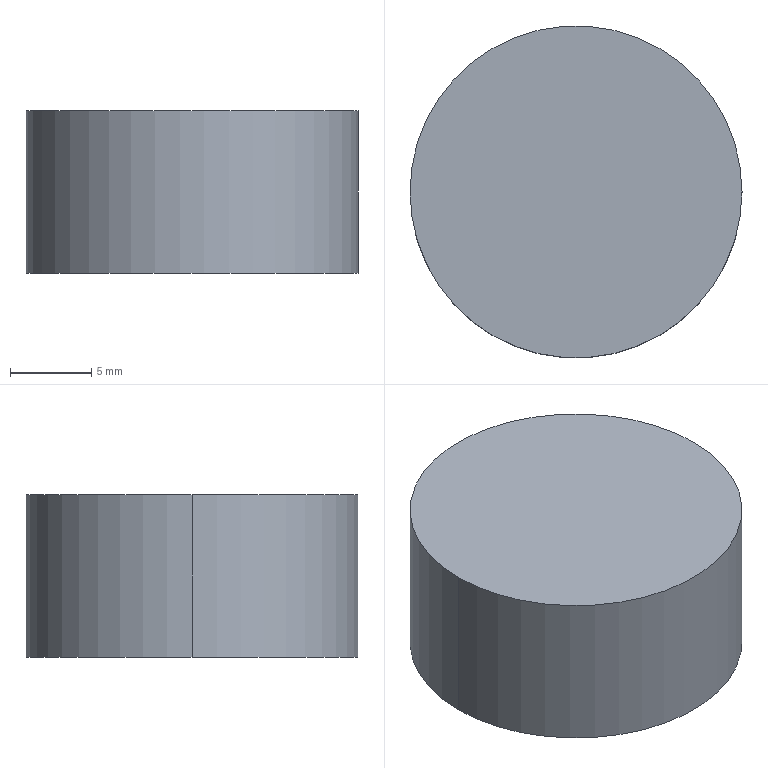Part | SolidWorks | features Extrusion 1 | 1 solid | 4 faces | box 20.49 x 20.49 x 10 mm | volume 3298 mm3 | cylinder 2 | plane 2 | commonest cylinder face diameters 20.49 x2
STEP:
#1=CARTESIAN_POINT('',(-128.618,112.983,10.));
#2=VERTEX_POINT('',#1);
#3=CARTESIAN_POINT('',(-149.109,112.983,10.));
#4=VERTEX_POINT('',#3);
#5=CARTESIAN_POINT('',(-138.863,112.983,10.));
#6=DIRECTION('',(0.,0.,1.));
#7=DIRECTION('',(1.,0.,0.));
#8=AXIS2_PLACEMENT_3D('',#5,#6,#7);
#9=CIRCLE('',#8,10.245);
#10=EDGE_CURVE('',#2,#4,#9,.T.);
#11=ORIENTED_EDGE('',*,*,#10,.F.);
#12=CARTESIAN_POINT('',(-128.618,112.983,0.));
#13=VERTEX_POINT('',#12);
#14=CARTESIAN_POINT('',(-128.618,112.983,10.));
#15=DIRECTION('',(0.,0.,-1.));
#16=VECTOR('',#15,1000.);
#17=LINE('',#14,#16);
#18=EDGE_CURVE('',#2,#13,#17,.T.);
#19=ORIENTED_EDGE('',*,*,#18,.T.);
#20=CARTESIAN_POINT('',(-149.109,112.983,0.));
#21=VERTEX_POINT('',#20);
#22=CARTESIAN_POINT('',(-138.863,112.983,0.));
#23=DIRECTION('',(0.,0.,1.));
#24=DIRECTION('',(1.,0.,0.));
#25=AXIS2_PLACEMENT_3D('',#22,#23,#24);
#26=CIRCLE('',#25,10.245);
#27=EDGE_CURVE('',#13,#21,#26,.T.);
#28=ORIENTED_EDGE('',*,*,#27,.T.);
#29=CARTESIAN_POINT('',(-149.109,112.983,10.));
#30=DIRECTION('',(0.,0.,-1.));
#31=VECTOR('',#30,1000.);
#32=LINE('',#29,#31);
#33=EDGE_CURVE('',#4,#21,#32,.T.);
#34=ORIENTED_EDGE('',*,*,#33,.F.);
#35=EDGE_LOOP('',(#11,#19,#28,#34));
#36=FACE_OUTER_BOUND('',#35,.T.);
#37=CARTESIAN_POINT('',(-138.863,112.983,10.));
#38=DIRECTION('',(0.,0.,-1.));
#39=DIRECTION('',(-1.,0.,0.));
#40=AXIS2_PLACEMENT_3D('',#37,#38,#39);
#41=CYLINDRICAL_SURFACE('',#40,10.245);
#42=ADVANCED_FACE('',(#36),#41,.T.);
#43=ORIENTED_EDGE('',*,*,#18,.F.);
#44=CARTESIAN_POINT('',(-138.863,112.983,10.));
#45=DIRECTION('',(0.,0.,1.));
#46=DIRECTION('',(1.,0.,0.));
#47=AXIS2_PLACEMENT_3D('',#44,#45,#46);
#48=CIRCLE('',#47,10.245);
#49=EDGE_CURVE('',#4,#2,#48,.T.);
#50=ORIENTED_EDGE('',*,*,#49,.F.);
#51=ORIENTED_EDGE('',*,*,#33,.T.);
#52=CARTESIAN_POINT('',(-138.863,112.983,0.));
#53=DIRECTION('',(0.,0.,1.));
#54=DIRECTION('',(1.,0.,0.));
#55=AXIS2_PLACEMENT_3D('',#52,#53,#54);
#56=CIRCLE('',#55,10.245);
#57=EDGE_CURVE('',#21,#13,#56,.T.);
#58=ORIENTED_EDGE('',*,*,#57,.T.);
#59=EDGE_LOOP('',(#43,#50,#51,#58));
#60=FACE_OUTER_BOUND('',#59,.T.);
#61=CARTESIAN_POINT('',(-138.863,112.983,10.));
#62=DIRECTION('',(0.,0.,-1.));
#63=DIRECTION('',(-1.,0.,0.));
#64=AXIS2_PLACEMENT_3D('',#61,#62,#63);
#65=CYLINDRICAL_SURFACE('',#64,10.245);
#66=ADVANCED_FACE('',(#60),#65,.T.);
#67=ORIENTED_EDGE('',*,*,#49,.T.);
#68=ORIENTED_EDGE('',*,*,#10,.T.);
#69=EDGE_LOOP('',(#67,#68));
#70=FACE_OUTER_BOUND('',#69,.T.);
#71=CARTESIAN_POINT('',(-138.863,112.983,10.));
#72=DIRECTION('',(0.,0.,1.));
#73=DIRECTION('',(1.,0.,0.));
#74=AXIS2_PLACEMENT_3D('',#71,#72,#73);
#75=PLANE('',#74);
#76=ADVANCED_FACE('',(#70),#75,.T.);
#77=ORIENTED_EDGE('',*,*,#57,.F.);
#78=ORIENTED_EDGE('',*,*,#27,.F.);
#79=EDGE_LOOP('',(#77,#78));
#80=FACE_OUTER_BOUND('',#79,.T.);
#81=CARTESIAN_POINT('',(-138.863,112.983,0.));
#82=DIRECTION('',(0.,0.,1.));
#83=DIRECTION('',(1.,0.,0.));
#84=AXIS2_PLACEMENT_3D('',#81,#82,#83);
#85=PLANE('',#84);
#86=ADVANCED_FACE('',(#80),#85,.F.);
#87=CLOSED_SHELL('',(#42,#66,#76,#86));
#88=MANIFOLD_SOLID_BREP('',#87);
#89=CARTESIAN_POINT('',(0.,0.,0.));
#90=DIRECTION('',(0.,0.,1.));
#91=DIRECTION('',(1.,0.,0.));
#92=AXIS2_PLACEMENT_3D('',#89,#90,#91);
#93=(LENGTH_UNIT()NAMED_UNIT(*)SI_UNIT(.MILLI.,.METRE.));
#94=UNCERTAINTY_MEASURE_WITH_UNIT(LENGTH_MEASURE(0.00001),#93,'','');
#95=(NAMED_UNIT(*)PLANE_ANGLE_UNIT()SI_UNIT($,.RADIAN.));
#96=(NAMED_UNIT(*)SI_UNIT($,.STERADIAN.)SOLID_ANGLE_UNIT());
#97=(GEOMETRIC_REPRESENTATION_CONTEXT(3)GLOBAL_UNCERTAINTY_ASSIGNED_CONTEXT((#94))GLOBAL_UNIT_ASSIGNED_CONTEXT((#93,#95,#96))REPRESENTATION_CONTEXT('',''));
#98=ADVANCED_BREP_SHAPE_REPRESENTATION('',(#88,#92),#97);